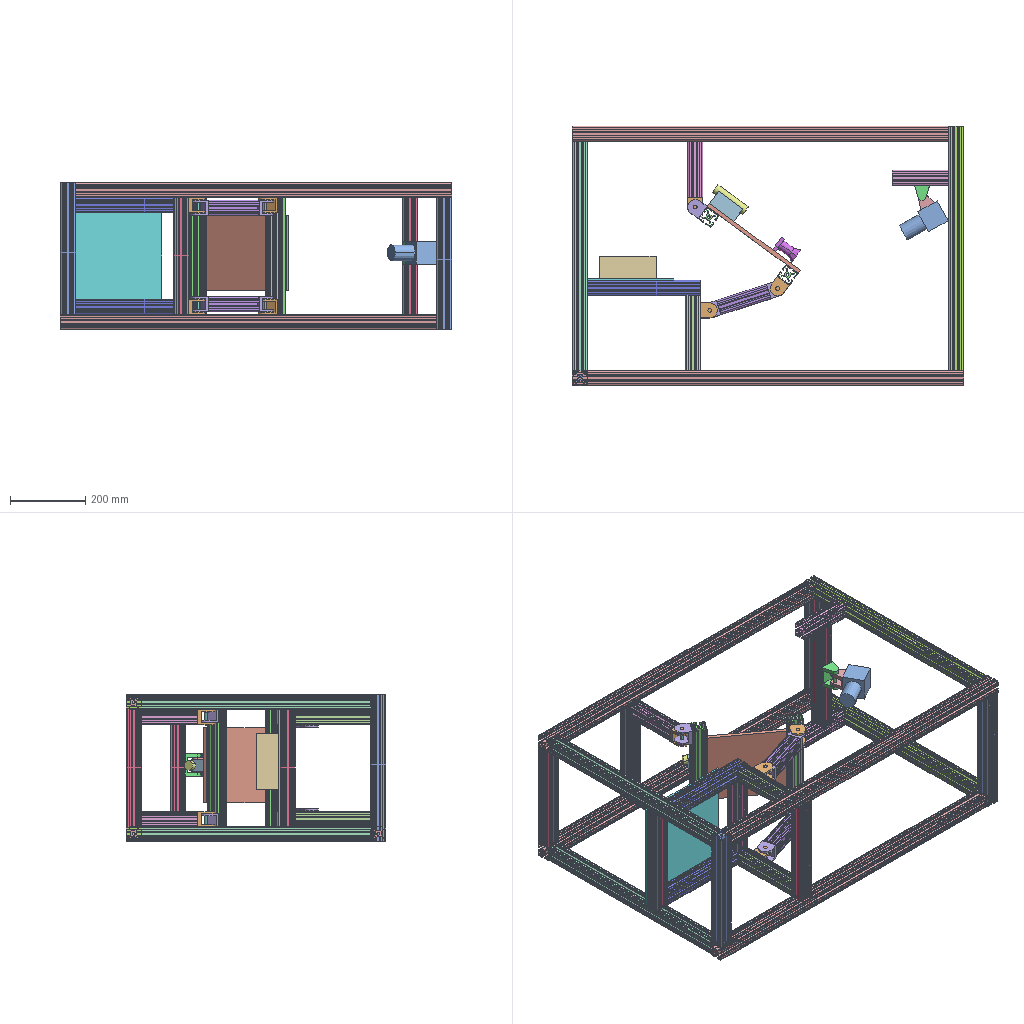Assembly | SolidWorks | 22 different items | 50 placed | box 1040 x 690 x 390 mm
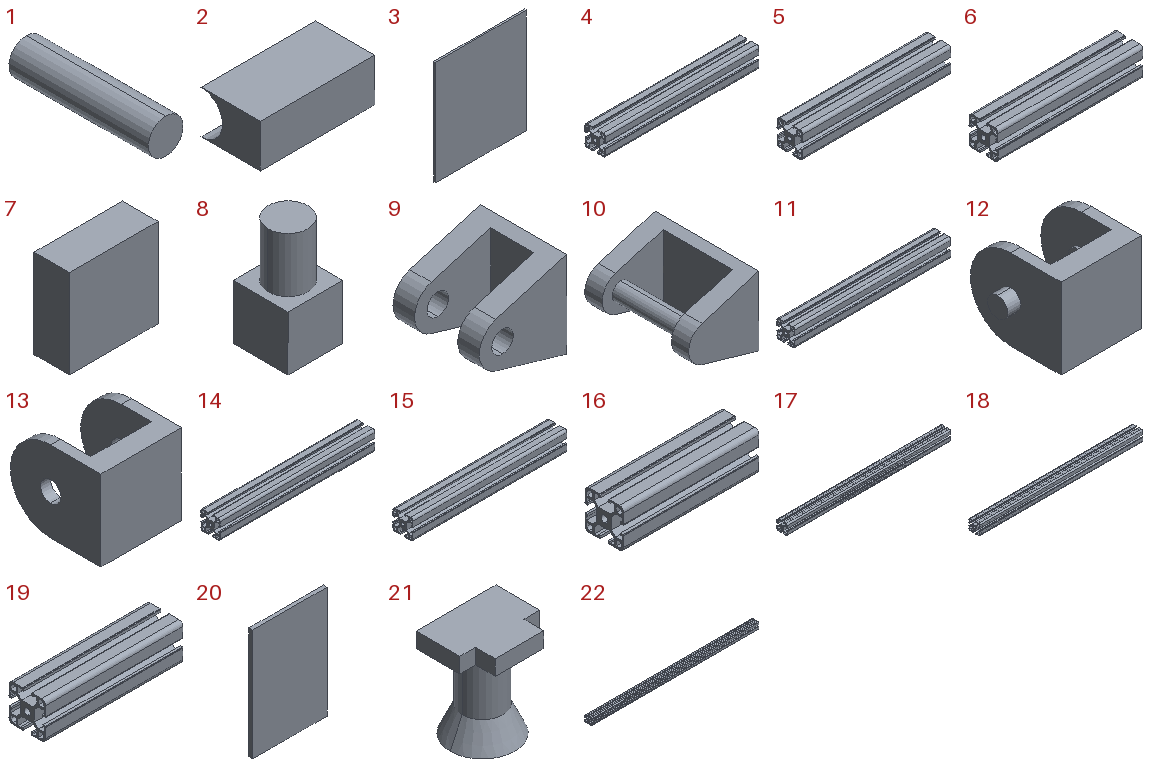Parts list (item | quantity | size | volume | features):
1 | x1 | 25 x 100 x 25 mm | 49087 mm3 | features Extrusion 1
2 | x1 | 80 x 41.33 x 30 mm | 70918 mm3 | features Extrusion 1, ICE 1
3 | x1 | 270 x 5 x 310 mm | 418500 mm3 | features Extrusion 1
4 | x2 | 300 x 40 x 40 mm | 172964 mm3 | features WeldMemberFeat 1, WeldmentFeature 1
5 | x1 | 230 x 40 x 40 mm | 132605 mm3 | features WeldMemberFeat 1, WeldmentFeature 1
6 | x2 | 200 x 40 x 40 mm | 115309 mm3 | features WeldMemberFeat 1, WeldmentFeature 1
7 | x1 | 150 x 60 x 150 mm | 1350000 mm3 | features Extrusion 1
8 | x1 | 60 x 60 x 120 mm | 307105 mm3 | features Extrusion 1, ICE 1
9 | x1 | 40.645 x 40 x 40 mm | 24880 mm3 | features ICE 2, Extrusion 1
10 | x1 | 40.645 x 60 x 40 mm | 33727 mm3 | features ICE 2, Extrusion 1
11 | x2 | 350 x 40 x 40 mm | 201791 mm3 | features WeldMemberFeat 1, WeldmentFeature 1
12 | x6 | 48 x 45 x 40 mm | 29911 mm3 | features ICE 4, MirrorPattern 2, Extrusion 1
13 | x6 | 40 x 45 x 40 mm | 27498 mm3 | features ICE 2, Extrusion 1, MirrorPattern 1
14 | x2 | 323 x 40 x 40 mm | 186224 mm3 | features WeldMemberFeat 1, WeldmentFeature 1
15 | x6 | 310 x 40 x 40 mm | 178729 mm3 | features WeldMemberFeat 1, WeldmentFeature 1
16 | x2 | 140 x 40 x 40 mm | 80716 mm3 | features WeldMemberFeat 1, WeldmentFeature 1
17 | x2 | 650 x 40 x 40 mm | 374755 mm3 | features WeldMemberFeat 1, WeldmentFeature 1
18 | x2 | 610 x 40 x 40 mm | 351693 mm3 | features WeldMemberFeat 1, WeldmentFeature 1
19 | x4 | 150 x 40 x 40 mm | 86482 mm3 | features WeldMemberFeat 1, WeldmentFeature 1
20 | x1 | 200 x 10 x 300 mm | 600000 mm3 | features Extrusion 1
21 | x1 | 51.992 x 45.152 x 61.712 mm | 54023 mm3 | features Extrusion 1, ICE 1, Revolution 1
22 | x4 | 1000 x 40 x 40 mm | 576545 mm3 | features WeldMemberFeat 1, WeldmentFeature 1
Mates (type | each side: item.copy, entity, surface, feature):
Coincident | 22.1 edge | 11.1 edge
Coincident | 22.1 face plane Aluminium profile 40 X 40B X R4.5(1) | 11.1 face plane Aluminium profile 40 X 40B X R4.5(1) | 2 times
Coincident | 11.1 edge | 22.2 edge
Coincident | 11.1 face plane Aluminium profile 40 X 40B X R4.5(1) | 22.2 face plane Aluminium profile 40 X 40B X R4.5(1)
Parallel | 22.1 face plane Aluminium profile 40 X 40B X R4.5(1) | 22.2 face plane Aluminium profile 40 X 40B X R4.5(1)
Coincident | 22.1 edge | 17.1 edge
Coincident | 22.1 face plane Aluminium profile 40 X 40B X R4.5(1) | 17.1 face plane Aluminium profile 40 X 40B X R4.5(1) | 2 times
Coincident | 11.1 edge | 17.2 edge
Coincident | 11.1 face plane Aluminium profile 40 X 40B X R4.5(1) | 17.2 face plane Aluminium profile 40 X 40B X R4.5(1) | 2 times
Coincident | 17.1 edge | 22.3 edge
Coincident | 17.1 face plane Aluminium profile 40 X 40B X R4.5(1) | 22.3 face plane Aluminium profile 40 X 40B X R4.5(1) | 3 times
Coincident | 17.2 edge | 22.4 edge
Coincident | 17.2 face plane Aluminium profile 40 X 40B X R4.5(1) | 22.4 face plane Aluminium profile 40 X 40B X R4.5(1) | 3 times
Coincident | 22.4 face plane Aluminium profile 40 X 40B X R4.5(1) | 19.1 face plane Aluminium profile 40 X 40B X R4.5(1)
Parallel | 19.2 edge | 19.1 edge
Coincident | 19.2 edge | 19.1 edge
Coincident | 19.2 edge | 12.1 select_type:24
Coincident | 19.2 face plane Aluminium profile 40 X 40B X R4.5(1) | 12.1 face plane Boss-Extrude1
Coincident | 12.1 edge | 13.1 edge
Coincident | 19.1 edge | 12.2 select_type:24
Coincident | 19.1 face plane Aluminium profile 40 X 40B X R4.5(1) | 12.2 face plane Boss-Extrude1
Coincident | 12.2 edge | 13.2 edge
Coincident | 13.1 edge | 13.2 edge
Coincident | 13.1 face plane Boss-Extrude1 | 14.1 face plane Aluminium profile 40 X 40B X R4.5(1) | 2 times
Coincident | 13.1 edge | 14.1 edge
Coincident | 17.2 face plane Aluminium profile 40 X 40B X R4.5(1) | 15.1 face plane Aluminium profile 40 X 40B X R4.5(1) | 3 times
Concentric | 2.1 face cylinder Boss-Extrude2 | 1.1 face cylinder Boss-Extrude1
DistanceDim | 1.1 face plane Boss-Extrude1 | 2.1 face plane Boss-Extrude1
DistanceDim | 21.1 face plane Boss-Extrude1 | 2.1 face plane Boss-Extrude1
Coincident | 22.1 face plane Aluminium profile 40 X 40B X R4.5(1) | 11.2 face plane Aluminium profile 40 X 40B X R4.5(1) | 3 times
Coincident | 22.3 face plane Aluminium profile 40 X 40B X R4.5(1) | 18.1 face plane Aluminium profile 40 X 40B X R4.5(1) | 3 times
Coincident | 22.4 face plane Aluminium profile 40 X 40B X R4.5(1) | 18.2 face plane Aluminium profile 40 X 40B X R4.5(1) | 3 times
Coincident | 22.4 face plane Aluminium profile 40 X 40B X R4.5(1) | 15.2 face plane Aluminium profile 40 X 40B X R4.5(1) | 3 times
Coincident | 14.1 face plane Aluminium profile 40 X 40B X R4.5(1) | 14.2 face plane Aluminium profile 40 X 40B X R4.5(1) | 2 times
Coincident | 14.1 face plane Aluminium profile 40 X 40B X R4.5(1) | 20.1 face plane Boss-Extrude1 | 2 times
Coincident | 14.2 face plane Aluminium profile 40 X 40B X R4.5(1) | 20.1 face plane Boss-Extrude1
Coincident | 2.1 face plane Boss-Extrude1 | 21.1 face plane Boss-Extrude1
Coincident | 21.1 face plane Boss-Extrude1 | 20.1 face plane Boss-Extrude1
Coincident | 2.1 face plane Boss-Extrude1 | 20.1 face plane Boss-Extrude1
DistanceDim | 2.1 face plane Boss-Extrude1 | 21.1 face plane Boss-Extrude1
DistanceDim | 21.1 face plane Boss-Extrude1 | 20.1 face plane Boss-Extrude1
Coincident | 13.2 face plane Boss-Extrude1 | 14.1 face plane Aluminium profile 40 X 40B X R4.5(1)
Coincident | 22.4 face plane Aluminium profile 40 X 40B X R4.5(1) | 15.3 face plane Aluminium profile 40 X 40B X R4.5(1)
Coincident | 22.3 face plane Aluminium profile 40 X 40B X R4.5(1) | 15.3 face plane Aluminium profile 40 X 40B X R4.5(1)
DistanceDim | 20.1 face plane Boss-Extrude1 | 14.1 face plane Aluminium profile 40 X 40B X R4.5(1)
Coincident | 19.2 face plane Aluminium profile 40 X 40B X R4.5(1) | 15.3 face plane Aluminium profile 40 X 40B X R4.5(1) | 2 times
Coincident | 22.1 face plane Aluminium profile 40 X 40B X R4.5(1) | 15.4 face plane Aluminium profile 40 X 40B X R4.5(1) | 2 times
Coincident | 14.2 face plane Aluminium profile 40 X 40B X R4.5(1) | 12.3 face plane Boss-Extrude1 | 2 times
DistanceDim | 12.3 face plane Boss-Extrude1 | 14.2 face plane Aluminium profile 40 X 40B X R4.5(1)
Coincident | 12.3 edge | 13.3 edge
Coincident | 18.1 face plane Aluminium profile 40 X 40B X R4.5(1) | 15.5 face plane Aluminium profile 40 X 40B X R4.5(1) | 2 times
DistanceDim | 15.5 face plane Aluminium profile 40 X 40B X R4.5(1) | 11.2 face plane Aluminium profile 40 X 40B X R4.5(1)
Coincident | 15.5 face plane Aluminium profile 40 X 40B X R4.5(1) | 4.1 face plane Aluminium profile 40 X 40B X R4.5(1) | 3 times
Coincident | 15.5 face plane Aluminium profile 40 X 40B X R4.5(1) | 4.2 face plane Aluminium profile 40 X 40B X R4.5(1) | 3 times
Coincident | 4.1 face plane Aluminium profile 40 X 40B X R4.5(1) | 6.1 face plane Aluminium profile 40 X 40B X R4.5(1) | 3 times
Coincident | 4.2 face plane Aluminium profile 40 X 40B X R4.5(1) | 6.2 face plane Aluminium profile 40 X 40B X R4.5(1) | 3 times
Coincident | 4.1 face plane Aluminium profile 40 X 40B X R4.5(1) | 5.1 face plane Aluminium profile 40 X 40B X R4.5(1) | 3 times
Coincident | 4.1 face plane Aluminium profile 40 X 40B X R4.5(1) | 3.1 face plane Boss-Extrude1 | 2 times
Coincident | 14.2 face plane Aluminium profile 40 X 40B X R4.5(1) | 12.4 face plane Boss-Extrude1 | 2 times
DistanceDim | 12.4 face plane Boss-Extrude1 | 14.2 face plane Aluminium profile 40 X 40B X R4.5(1)
Coincident | 13.4 edge | 12.4 edge
Coincident | 6.1 face plane Aluminium profile 40 X 40B X R4.5(1) | 12.5 face plane Boss-Extrude1 | 2 times
Coincident | 12.5 edge | 13.5 edge
DistanceDim | 12.5 face plane Boss-Extrude1 | 15.4 face plane Aluminium profile 40 X 40B X R4.5(1)
Coincident | 13.5 face plane Boss-Extrude1 | 16.1 face plane Aluminium profile 40 X 40B X R4.5(1) | 3 times
Coincident | 13.3 face plane Boss-Extrude1 | 16.1 face plane Aluminium profile 40 X 40B X R4.5(1) | 2 times
Coincident | 6.2 face plane Aluminium profile 40 X 40B X R4.5(1) | 12.6 face plane Boss-Extrude1 | 2 times
Coincident | 12.5 face plane Boss-Extrude1 | 12.6 face plane Boss-Extrude1
Coincident | 12.6 edge | 13.6 edge
Coincident | 13.6 face plane Boss-Extrude1 | 16.2 face plane Aluminium profile 40 X 40B X R4.5(1) | 3 times
Coincident | 13.4 face plane Boss-Extrude1 | 16.2 face plane Aluminium profile 40 X 40B X R4.5(1)
Coincident | 15.5 face plane Aluminium profile 40 X 40B X R4.5(1) | 3.1 face plane Boss-Extrude1
Coincident | 15.4 face plane Aluminium profile 40 X 40B X R4.5(1) | 5.1 face plane Aluminium profile 40 X 40B X R4.5(1)
Coincident | 17.2 face plane Aluminium profile 40 X 40B X R4.5(1) | 19.3 face plane Aluminium profile 40 X 40B X R4.5(1) | 2 times
Coincident | 17.1 face plane Aluminium profile 40 X 40B X R4.5(1) | 19.4 face plane Aluminium profile 40 X 40B X R4.5(1) | 2 times
Coincident | 19.3 face plane Aluminium profile 40 X 40B X R4.5(1) | 19.4 face plane Aluminium profile 40 X 40B X R4.5(1)
Coincident | 19.4 face plane Aluminium profile 40 X 40B X R4.5(1) | 15.6 face plane Aluminium profile 40 X 40B X R4.5(1) | 2 times
Coincident | 15.6 face plane Aluminium profile 40 X 40B X R4.5(1) | 10.1 face plane Boss-Extrude1
Coincident | 15.6 face plane Aluminium profile 40 X 40B X R4.5(1) | 10.1 edge
Coincident | 10.1 face plane Cut-Extrude1 | 9.1 face plane Boss-Extrude1
Concentric | 10.1 face cylinder Boss-Extrude2 | 9.1 face cylinder Cut-Extrude2
Coincident | 9.1 face plane Boss-Extrude1 | 8.1 face plane Boss-Extrude1
DistanceDim | 8.1 face plane Boss-Extrude1 | 9.1 edge
DistanceDim | 8.1 edge | 9.1 edge